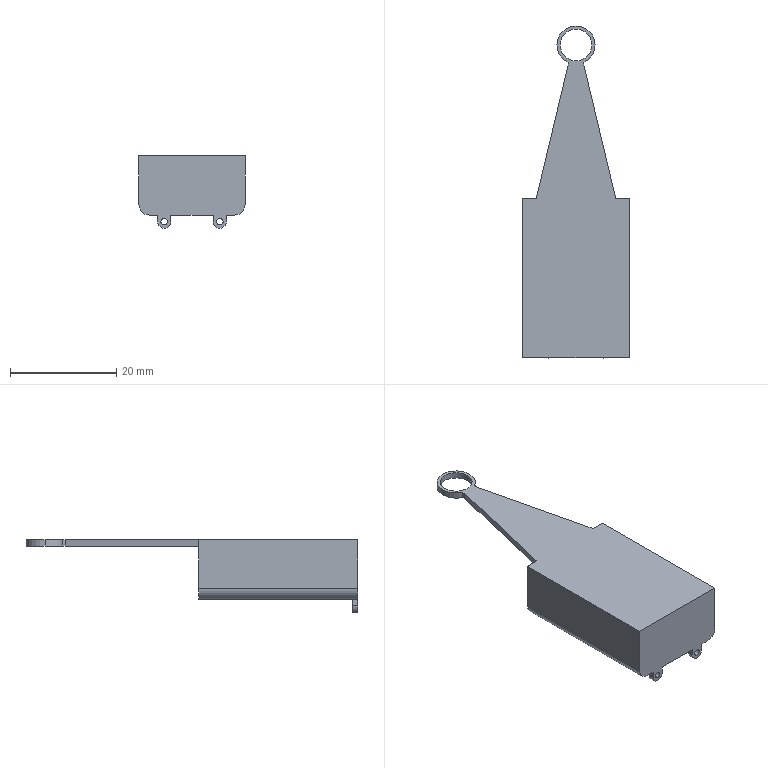Part | SolidWorks | features ICE 2, Extrusion 1, Fillet 1 | 1 solid | 32 faces | box 20 x 62.6 x 13.7 mm | volume 6966 mm3 | plane 17 | cylinder 15 | commonest cylinder face diameters 1.2 x4 2.5 x4 7.2 x3 4 x2 6 x2
STEP:
#1=CARTESIAN_POINT('',(5.25,1.,-6.25));
#2=VERTEX_POINT('',#1);
#3=CARTESIAN_POINT('',(5.25,1.,-7.45));
#4=VERTEX_POINT('',#3);
#5=CARTESIAN_POINT('',(5.25,1.,-6.85));
#6=DIRECTION('',(0.,-1.,0.));
#7=DIRECTION('',(0.,0.,1.));
#8=AXIS2_PLACEMENT_3D('',#5,#6,#7);
#9=CIRCLE('',#8,0.6);
#10=EDGE_CURVE('',#2,#4,#9,.T.);
#11=ORIENTED_EDGE('',*,*,#10,.F.);
#12=CARTESIAN_POINT('',(5.25,0.,-6.25));
#13=VERTEX_POINT('',#12);
#14=CARTESIAN_POINT('',(5.25,1.,-6.25));
#15=DIRECTION('',(0.,-1.,0.));
#16=VECTOR('',#15,1000.);
#17=LINE('',#14,#16);
#18=EDGE_CURVE('',#2,#13,#17,.T.);
#19=ORIENTED_EDGE('',*,*,#18,.T.);
#20=CARTESIAN_POINT('',(5.25,0.,-7.45));
#21=VERTEX_POINT('',#20);
#22=CARTESIAN_POINT('',(5.25,0.,-6.85));
#23=DIRECTION('',(0.,-1.,0.));
#24=DIRECTION('',(0.,0.,1.));
#25=AXIS2_PLACEMENT_3D('',#22,#23,#24);
#26=CIRCLE('',#25,0.6);
#27=EDGE_CURVE('',#13,#21,#26,.T.);
#28=ORIENTED_EDGE('',*,*,#27,.T.);
#29=CARTESIAN_POINT('',(5.25,1.,-7.45));
#30=DIRECTION('',(0.,-1.,0.));
#31=VECTOR('',#30,1000.);
#32=LINE('',#29,#31);
#33=EDGE_CURVE('',#4,#21,#32,.T.);
#34=ORIENTED_EDGE('',*,*,#33,.F.);
#35=EDGE_LOOP('',(#11,#19,#28,#34));
#36=FACE_OUTER_BOUND('',#35,.T.);
#37=CARTESIAN_POINT('',(5.25,1.,-6.85));
#38=DIRECTION('',(0.,-1.,0.));
#39=DIRECTION('',(0.,0.,-1.));
#40=AXIS2_PLACEMENT_3D('',#37,#38,#39);
#41=CYLINDRICAL_SURFACE('',#40,0.6);
#42=ADVANCED_FACE('',(#36),#41,.F.);
#43=CARTESIAN_POINT('',(4.,1.,-6.85));
#44=VERTEX_POINT('',#43);
#45=CARTESIAN_POINT('',(5.25,1.,-8.1));
#46=VERTEX_POINT('',#45);
#47=CARTESIAN_POINT('',(5.25,1.,-6.85));
#48=DIRECTION('',(0.,-1.,0.));
#49=DIRECTION('',(0.,0.,1.));
#50=AXIS2_PLACEMENT_3D('',#47,#48,#49);
#51=CIRCLE('',#50,1.25);
#52=EDGE_CURVE('',#44,#46,#51,.T.);
#53=ORIENTED_EDGE('',*,*,#52,.T.);
#54=CARTESIAN_POINT('',(5.25,0.,-8.1));
#55=VERTEX_POINT('',#54);
#56=CARTESIAN_POINT('',(5.25,1.,-8.1));
#57=DIRECTION('',(0.,-1.,0.));
#58=VECTOR('',#57,1000.);
#59=LINE('',#56,#58);
#60=EDGE_CURVE('',#46,#55,#59,.T.);
#61=ORIENTED_EDGE('',*,*,#60,.T.);
#62=CARTESIAN_POINT('',(4.,0.,-6.85));
#63=VERTEX_POINT('',#62);
#64=CARTESIAN_POINT('',(5.25,0.,-6.85));
#65=DIRECTION('',(0.,-1.,0.));
#66=DIRECTION('',(0.,0.,1.));
#67=AXIS2_PLACEMENT_3D('',#64,#65,#66);
#68=CIRCLE('',#67,1.25);
#69=EDGE_CURVE('',#63,#55,#68,.T.);
#70=ORIENTED_EDGE('',*,*,#69,.F.);
#71=CARTESIAN_POINT('',(4.,1.,-6.85));
#72=DIRECTION('',(0.,-1.,0.));
#73=VECTOR('',#72,1000.);
#74=LINE('',#71,#73);
#75=EDGE_CURVE('',#44,#63,#74,.T.);
#76=ORIENTED_EDGE('',*,*,#75,.F.);
#77=EDGE_LOOP('',(#53,#61,#70,#76));
#78=FACE_OUTER_BOUND('',#77,.T.);
#79=CARTESIAN_POINT('',(5.25,1.,-6.85));
#80=DIRECTION('',(0.,-1.,0.));
#81=DIRECTION('',(0.,0.,-1.));
#82=AXIS2_PLACEMENT_3D('',#79,#80,#81);
#83=CYLINDRICAL_SURFACE('',#82,1.25);
#84=ADVANCED_FACE('',(#78),#83,.T.);
#85=CARTESIAN_POINT('',(-5.25,1.,-6.25));
#86=VERTEX_POINT('',#85);
#87=CARTESIAN_POINT('',(-5.25,1.,-7.45));
#88=VERTEX_POINT('',#87);
#89=CARTESIAN_POINT('',(-5.25,1.,-6.85));
#90=DIRECTION('',(0.,-1.,0.));
#91=DIRECTION('',(0.,0.,-1.));
#92=AXIS2_PLACEMENT_3D('',#89,#90,#91);
#93=CIRCLE('',#92,0.6);
#94=EDGE_CURVE('',#86,#88,#93,.T.);
#95=ORIENTED_EDGE('',*,*,#94,.F.);
#96=CARTESIAN_POINT('',(-5.25,0.,-6.25));
#97=VERTEX_POINT('',#96);
#98=CARTESIAN_POINT('',(-5.25,1.,-6.25));
#99=DIRECTION('',(0.,-1.,0.));
#100=VECTOR('',#99,1000.);
#101=LINE('',#98,#100);
#102=EDGE_CURVE('',#86,#97,#101,.T.);
#103=ORIENTED_EDGE('',*,*,#102,.T.);
#104=CARTESIAN_POINT('',(-5.25,0.,-7.45));
#105=VERTEX_POINT('',#104);
#106=CARTESIAN_POINT('',(-5.25,0.,-6.85));
#107=DIRECTION('',(0.,-1.,0.));
#108=DIRECTION('',(0.,0.,-1.));
#109=AXIS2_PLACEMENT_3D('',#106,#107,#108);
#110=CIRCLE('',#109,0.6);
#111=EDGE_CURVE('',#97,#105,#110,.T.);
#112=ORIENTED_EDGE('',*,*,#111,.T.);
#113=CARTESIAN_POINT('',(-5.25,1.,-7.45));
#114=DIRECTION('',(0.,-1.,0.));
#115=VECTOR('',#114,1000.);
#116=LINE('',#113,#115);
#117=EDGE_CURVE('',#88,#105,#116,.T.);
#118=ORIENTED_EDGE('',*,*,#117,.F.);
#119=EDGE_LOOP('',(#95,#103,#112,#118));
#120=FACE_OUTER_BOUND('',#119,.T.);
#121=CARTESIAN_POINT('',(-5.25,1.,-6.85));
#122=DIRECTION('',(0.,-1.,0.));
#123=DIRECTION('',(0.,0.,-1.));
#124=AXIS2_PLACEMENT_3D('',#121,#122,#123);
#125=CYLINDRICAL_SURFACE('',#124,0.6);
#126=ADVANCED_FACE('',(#120),#125,.F.);
#127=CARTESIAN_POINT('',(-6.5,1.,-6.85));
#128=VERTEX_POINT('',#127);
#129=CARTESIAN_POINT('',(-5.25,1.,-8.1));
#130=VERTEX_POINT('',#129);
#131=CARTESIAN_POINT('',(-5.25,1.,-6.85));
#132=DIRECTION('',(0.,-1.,0.));
#133=DIRECTION('',(0.,0.,-1.));
#134=AXIS2_PLACEMENT_3D('',#131,#132,#133);
#135=CIRCLE('',#134,1.25);
#136=EDGE_CURVE('',#128,#130,#135,.T.);
#137=ORIENTED_EDGE('',*,*,#136,.T.);
#138=CARTESIAN_POINT('',(-5.25,0.,-8.1));
#139=VERTEX_POINT('',#138);
#140=CARTESIAN_POINT('',(-5.25,1.,-8.1));
#141=DIRECTION('',(0.,-1.,0.));
#142=VECTOR('',#141,1000.);
#143=LINE('',#140,#142);
#144=EDGE_CURVE('',#130,#139,#143,.T.);
#145=ORIENTED_EDGE('',*,*,#144,.T.);
#146=CARTESIAN_POINT('',(-6.5,0.,-6.85));
#147=VERTEX_POINT('',#146);
#148=CARTESIAN_POINT('',(-5.25,0.,-6.85));
#149=DIRECTION('',(0.,-1.,0.));
#150=DIRECTION('',(0.,0.,-1.));
#151=AXIS2_PLACEMENT_3D('',#148,#149,#150);
#152=CIRCLE('',#151,1.25);
#153=EDGE_CURVE('',#147,#139,#152,.T.);
#154=ORIENTED_EDGE('',*,*,#153,.F.);
#155=CARTESIAN_POINT('',(-6.5,1.,-6.85));
#156=DIRECTION('',(0.,-1.,0.));
#157=VECTOR('',#156,1000.);
#158=LINE('',#155,#157);
#159=EDGE_CURVE('',#128,#147,#158,.T.);
#160=ORIENTED_EDGE('',*,*,#159,.F.);
#161=EDGE_LOOP('',(#137,#145,#154,#160));
#162=FACE_OUTER_BOUND('',#161,.T.);
#163=CARTESIAN_POINT('',(-5.25,1.,-6.85));
#164=DIRECTION('',(0.,-1.,0.));
#165=DIRECTION('',(0.,0.,-1.));
#166=AXIS2_PLACEMENT_3D('',#163,#164,#165);
#167=CYLINDRICAL_SURFACE('',#166,1.25);
#168=ADVANCED_FACE('',(#162),#167,.T.);
#169=CARTESIAN_POINT('',(-3.,59.,4.4));
#170=VERTEX_POINT('',#169);
#171=CARTESIAN_POINT('',(3.,59.,4.4));
#172=VERTEX_POINT('',#171);
#173=CARTESIAN_POINT('',(0.,59.,4.4));
#174=DIRECTION('',(0.,0.,1.));
#175=DIRECTION('',(1.,0.,0.));
#176=AXIS2_PLACEMENT_3D('',#173,#174,#175);
#177=CIRCLE('',#176,3.);
#178=EDGE_CURVE('',#170,#172,#177,.T.);
#179=ORIENTED_EDGE('',*,*,#178,.F.);
#180=CARTESIAN_POINT('',(-3.,59.,5.6));
#181=VERTEX_POINT('',#180);
#182=CARTESIAN_POINT('',(-3.,59.,4.4));
#183=DIRECTION('',(0.,0.,1.));
#184=VECTOR('',#183,1000.);
#185=LINE('',#182,#184);
#186=EDGE_CURVE('',#170,#181,#185,.T.);
#187=ORIENTED_EDGE('',*,*,#186,.T.);
#188=CARTESIAN_POINT('',(3.,59.,5.6));
#189=VERTEX_POINT('',#188);
#190=CARTESIAN_POINT('',(0.,59.,5.6));
#191=DIRECTION('',(0.,0.,1.));
#192=DIRECTION('',(1.,0.,0.));
#193=AXIS2_PLACEMENT_3D('',#190,#191,#192);
#194=CIRCLE('',#193,3.);
#195=EDGE_CURVE('',#181,#189,#194,.T.);
#196=ORIENTED_EDGE('',*,*,#195,.T.);
#197=CARTESIAN_POINT('',(3.,59.,4.4));
#198=DIRECTION('',(0.,0.,1.));
#199=VECTOR('',#198,1000.);
#200=LINE('',#197,#199);
#201=EDGE_CURVE('',#172,#189,#200,.T.);
#202=ORIENTED_EDGE('',*,*,#201,.F.);
#203=EDGE_LOOP('',(#179,#187,#196,#202));
#204=FACE_OUTER_BOUND('',#203,.T.);
#205=CARTESIAN_POINT('',(0.,59.,4.4));
#206=DIRECTION('',(0.,0.,1.));
#207=DIRECTION('',(1.,0.,0.));
#208=AXIS2_PLACEMENT_3D('',#205,#206,#207);
#209=CYLINDRICAL_SURFACE('',#208,3.);
#210=ADVANCED_FACE('',(#204),#209,.F.);
#211=CARTESIAN_POINT('',(3.6,59.,4.4));
#212=VERTEX_POINT('',#211);
#213=CARTESIAN_POINT('',(-3.6,59.,4.4));
#214=VERTEX_POINT('',#213);
#215=CARTESIAN_POINT('',(0.,59.,4.4));
#216=DIRECTION('',(0.,0.,1.));
#217=DIRECTION('',(1.,0.,0.));
#218=AXIS2_PLACEMENT_3D('',#215,#216,#217);
#219=CIRCLE('',#218,3.6);
#220=EDGE_CURVE('',#212,#214,#219,.T.);
#221=ORIENTED_EDGE('',*,*,#220,.T.);
#222=CARTESIAN_POINT('',(-3.6,59.,5.6));
#223=VERTEX_POINT('',#222);
#224=CARTESIAN_POINT('',(-3.6,59.,4.4));
#225=DIRECTION('',(0.,0.,1.));
#226=VECTOR('',#225,1000.);
#227=LINE('',#224,#226);
#228=EDGE_CURVE('',#214,#223,#227,.T.);
#229=ORIENTED_EDGE('',*,*,#228,.T.);
#230=CARTESIAN_POINT('',(3.6,59.,5.6));
#231=VERTEX_POINT('',#230);
#232=CARTESIAN_POINT('',(0.,59.,5.6));
#233=DIRECTION('',(0.,0.,1.));
#234=DIRECTION('',(1.,0.,0.));
#235=AXIS2_PLACEMENT_3D('',#232,#233,#234);
#236=CIRCLE('',#235,3.6);
#237=EDGE_CURVE('',#231,#223,#236,.T.);
#238=ORIENTED_EDGE('',*,*,#237,.F.);
#239=CARTESIAN_POINT('',(3.6,59.,4.4));
#240=DIRECTION('',(0.,0.,1.));
#241=VECTOR('',#240,1000.);
#242=LINE('',#239,#241);
#243=EDGE_CURVE('',#212,#231,#242,.T.);
#244=ORIENTED_EDGE('',*,*,#243,.F.);
#245=EDGE_LOOP('',(#221,#229,#238,#244));
#246=FACE_OUTER_BOUND('',#245,.T.);
#247=CARTESIAN_POINT('',(0.,59.,4.4));
#248=DIRECTION('',(0.,0.,1.));
#249=DIRECTION('',(1.,0.,0.));
#250=AXIS2_PLACEMENT_3D('',#247,#248,#249);
#251=CYLINDRICAL_SURFACE('',#250,3.6);
#252=ADVANCED_FACE('',(#246),#251,.T.);
#253=CARTESIAN_POINT('',(1.5,55.727,4.4));
#254=VERTEX_POINT('',#253);
#255=CARTESIAN_POINT('',(0.,59.,4.4));
#256=DIRECTION('',(0.,0.,1.));
#257=DIRECTION('',(1.,0.,0.));
#258=AXIS2_PLACEMENT_3D('',#255,#256,#257);
#259=CIRCLE('',#258,3.6);
#260=EDGE_CURVE('',#254,#212,#259,.T.);
#261=ORIENTED_EDGE('',*,*,#260,.T.);
#262=ORIENTED_EDGE('',*,*,#243,.T.);
#263=CARTESIAN_POINT('',(1.5,55.727,5.6));
#264=VERTEX_POINT('',#263);
#265=CARTESIAN_POINT('',(0.,59.,5.6));
#266=DIRECTION('',(0.,0.,1.));
#267=DIRECTION('',(1.,0.,0.));
#268=AXIS2_PLACEMENT_3D('',#265,#266,#267);
#269=CIRCLE('',#268,3.6);
#270=EDGE_CURVE('',#264,#231,#269,.T.);
#271=ORIENTED_EDGE('',*,*,#270,.F.);
#272=CARTESIAN_POINT('',(1.5,55.727,4.4));
#273=DIRECTION('',(0.,0.,1.));
#274=VECTOR('',#273,1000.);
#275=LINE('',#272,#274);
#276=EDGE_CURVE('',#254,#264,#275,.T.);
#277=ORIENTED_EDGE('',*,*,#276,.F.);
#278=EDGE_LOOP('',(#261,#262,#271,#277));
#279=FACE_OUTER_BOUND('',#278,.T.);
#280=CARTESIAN_POINT('',(0.,59.,4.4));
#281=DIRECTION('',(0.,0.,1.));
#282=DIRECTION('',(1.,0.,0.));
#283=AXIS2_PLACEMENT_3D('',#280,#281,#282);
#284=CYLINDRICAL_SURFACE('',#283,3.6);
#285=ADVANCED_FACE('',(#279),#284,.T.);
#286=CARTESIAN_POINT('',(10.,0.,5.6));
#287=VERTEX_POINT('',#286);
#288=CARTESIAN_POINT('',(10.,0.,-3.6));
#289=VERTEX_POINT('',#288);
#290=CARTESIAN_POINT('',(10.,0.,-5.6));
#291=DIRECTION('',(0.,0.,-1.));
#292=VECTOR('',#291,1000.);
#293=LINE('',#290,#292);
#294=EDGE_CURVE('',#287,#289,#293,.T.);
#295=ORIENTED_EDGE('',*,*,#294,.T.);
#296=CARTESIAN_POINT('',(10.,30.,-3.6));
#297=VERTEX_POINT('',#296);
#298=CARTESIAN_POINT('',(10.,30.,-3.6));
#299=DIRECTION('',(0.,1.,0.));
#300=VECTOR('',#299,1000.);
#301=LINE('',#298,#300);
#302=EDGE_CURVE('',#289,#297,#301,.T.);
#303=ORIENTED_EDGE('',*,*,#302,.T.);
#304=CARTESIAN_POINT('',(10.,30.,5.6));
#305=VERTEX_POINT('',#304);
#306=CARTESIAN_POINT('',(10.,30.,-5.6));
#307=DIRECTION('',(0.,0.,-1.));
#308=VECTOR('',#307,1000.);
#309=LINE('',#306,#308);
#310=EDGE_CURVE('',#305,#297,#309,.T.);
#311=ORIENTED_EDGE('',*,*,#310,.F.);
#312=CARTESIAN_POINT('',(10.,30.,5.6));
#313=DIRECTION('',(0.,-1.,0.));
#314=VECTOR('',#313,1000.);
#315=LINE('',#312,#314);
#316=EDGE_CURVE('',#305,#287,#315,.T.);
#317=ORIENTED_EDGE('',*,*,#316,.T.);
#318=EDGE_LOOP('',(#295,#303,#311,#317));
#319=FACE_OUTER_BOUND('',#318,.T.);
#320=CARTESIAN_POINT('',(10.,30.,-5.6));
#321=DIRECTION('',(-1.,0.,0.));
#322=DIRECTION('',(0.,0.,1.));
#323=AXIS2_PLACEMENT_3D('',#320,#321,#322);
#324=PLANE('',#323);
#325=ADVANCED_FACE('',(#319),#324,.F.);
#326=CARTESIAN_POINT('',(8.,0.,-5.6));
#327=VERTEX_POINT('',#326);
#328=CARTESIAN_POINT('',(6.5,0.,-5.6));
#329=VERTEX_POINT('',#328);
#330=CARTESIAN_POINT('',(-10.,0.,-5.6));
#331=DIRECTION('',(-1.,0.,0.));
#332=VECTOR('',#331,1000.);
#333=LINE('',#330,#332);
#334=EDGE_CURVE('',#327,#329,#333,.T.);
#335=ORIENTED_EDGE('',*,*,#334,.T.);
#336=CARTESIAN_POINT('',(6.5,1.,-5.6));
#337=VERTEX_POINT('',#336);
#338=CARTESIAN_POINT('',(6.5,1.,-5.6));
#339=DIRECTION('',(0.,-1.,0.));
#340=VECTOR('',#339,1000.);
#341=LINE('',#338,#340);
#342=EDGE_CURVE('',#337,#329,#341,.T.);
#343=ORIENTED_EDGE('',*,*,#342,.F.);
#344=CARTESIAN_POINT('',(4.,1.,-5.6));
#345=VERTEX_POINT('',#344);
#346=CARTESIAN_POINT('',(6.5,1.,-5.6));
#347=DIRECTION('',(-1.,0.,0.));
#348=VECTOR('',#347,1000.);
#349=LINE('',#346,#348);
#350=EDGE_CURVE('',#337,#345,#349,.T.);
#351=ORIENTED_EDGE('',*,*,#350,.T.);
#352=CARTESIAN_POINT('',(4.,0.,-5.6));
#353=VERTEX_POINT('',#352);
#354=CARTESIAN_POINT('',(4.,1.,-5.6));
#355=DIRECTION('',(0.,-1.,0.));
#356=VECTOR('',#355,1000.);
#357=LINE('',#354,#356);
#358=EDGE_CURVE('',#345,#353,#357,.T.);
#359=ORIENTED_EDGE('',*,*,#358,.T.);
#360=CARTESIAN_POINT('',(-4.,0.,-5.6));
#361=VERTEX_POINT('',#360);
#362=CARTESIAN_POINT('',(-10.,0.,-5.6));
#363=DIRECTION('',(-1.,0.,0.));
#364=VECTOR('',#363,1000.);
#365=LINE('',#362,#364);
#366=EDGE_CURVE('',#353,#361,#365,.T.);
#367=ORIENTED_EDGE('',*,*,#366,.T.);
#368=CARTESIAN_POINT('',(-4.,1.,-5.6));
#369=VERTEX_POINT('',#368);
#370=CARTESIAN_POINT('',(-4.,1.,-5.6));
#371=DIRECTION('',(0.,-1.,0.));
#372=VECTOR('',#371,1000.);
#373=LINE('',#370,#372);
#374=EDGE_CURVE('',#369,#361,#373,.T.);
#375=ORIENTED_EDGE('',*,*,#374,.F.);
#376=CARTESIAN_POINT('',(-6.5,1.,-5.6));
#377=VERTEX_POINT('',#376);
#378=CARTESIAN_POINT('',(-6.5,1.,-5.6));
#379=DIRECTION('',(-1.,0.,0.));
#380=VECTOR('',#379,1000.);
#381=LINE('',#378,#380);
#382=EDGE_CURVE('',#369,#377,#381,.T.);
#383=ORIENTED_EDGE('',*,*,#382,.T.);
#384=CARTESIAN_POINT('',(-6.5,0.,-5.6));
#385=VERTEX_POINT('',#384);
#386=CARTESIAN_POINT('',(-6.5,1.,-5.6));
#387=DIRECTION('',(0.,-1.,0.));
#388=VECTOR('',#387,1000.);
#389=LINE('',#386,#388);
#390=EDGE_CURVE('',#377,#385,#389,.T.);
#391=ORIENTED_EDGE('',*,*,#390,.T.);
#392=CARTESIAN_POINT('',(-8.,0.,-5.6));
#393=VERTEX_POINT('',#392);
#394=CARTESIAN_POINT('',(-10.,0.,-5.6));
#395=DIRECTION('',(-1.,0.,0.));
#396=VECTOR('',#395,1000.);
#397=LINE('',#394,#396);
#398=EDGE_CURVE('',#385,#393,#397,.T.);
#399=ORIENTED_EDGE('',*,*,#398,.T.);
#400=CARTESIAN_POINT('',(-8.,30.,-5.6));
#401=VERTEX_POINT('',#400);
#402=CARTESIAN_POINT('',(-8.,30.,-5.6));
#403=DIRECTION('',(0.,1.,0.));
#404=VECTOR('',#403,1000.);
#405=LINE('',#402,#404);
#406=EDGE_CURVE('',#393,#401,#405,.T.);
#407=ORIENTED_EDGE('',*,*,#406,.T.);
#408=CARTESIAN_POINT('',(8.,30.,-5.6));
#409=VERTEX_POINT('',#408);
#410=CARTESIAN_POINT('',(-10.,30.,-5.6));
#411=DIRECTION('',(-1.,0.,0.));
#412=VECTOR('',#411,1000.);
#413=LINE('',#410,#412);
#414=EDGE_CURVE('',#409,#401,#413,.T.);
#415=ORIENTED_EDGE('',*,*,#414,.F.);
#416=CARTESIAN_POINT('',(8.,30.,-5.6));
#417=DIRECTION('',(0.,-1.,0.));
#418=VECTOR('',#417,1000.);
#419=LINE('',#416,#418);
#420=EDGE_CURVE('',#409,#327,#419,.T.);
#421=ORIENTED_EDGE('',*,*,#420,.T.);
#422=EDGE_LOOP('',(#335,#343,#351,#359,#367,#375,#383,#391,#399,#407,#415,#421));
#423=FACE_OUTER_BOUND('',#422,.T.);
#424=CARTESIAN_POINT('',(-10.,30.,-5.6));
#425=DIRECTION('',(0.,0.,1.));
#426=DIRECTION('',(1.,0.,0.));
#427=AXIS2_PLACEMENT_3D('',#424,#425,#426);
#428=PLANE('',#427);
#429=ADVANCED_FACE('',(#423),#428,.F.);
#430=CARTESIAN_POINT('',(-10.,30.,-3.6));
#431=VERTEX_POINT('',#430);
#432=CARTESIAN_POINT('',(-10.,30.,5.6));
#433=VERTEX_POINT('',#432);
#434=CARTESIAN_POINT('',(-10.,30.,-5.6));
#435=DIRECTION('',(0.,0.,1.));
#436=VECTOR('',#435,1000.);
#437=LINE('',#434,#436);
#438=EDGE_CURVE('',#431,#433,#437,.T.);
#439=ORIENTED_EDGE('',*,*,#438,.F.);
#440=CARTESIAN_POINT('',(-10.,0.,-3.6));
#441=VERTEX_POINT('',#440);
#442=CARTESIAN_POINT('',(-10.,30.,-3.6));
#443=DIRECTION('',(0.,-1.,0.));
#444=VECTOR('',#443,1000.);
#445=LINE('',#442,#444);
#446=EDGE_CURVE('',#431,#441,#445,.T.);
#447=ORIENTED_EDGE('',*,*,#446,.T.);
#448=CARTESIAN_POINT('',(-10.,0.,5.6));
#449=VERTEX_POINT('',#448);
#450=CARTESIAN_POINT('',(-10.,0.,-5.6));
#451=DIRECTION('',(0.,0.,1.));
#452=VECTOR('',#451,1000.);
#453=LINE('',#450,#452);
#454=EDGE_CURVE('',#441,#449,#453,.T.);
#455=ORIENTED_EDGE('',*,*,#454,.T.);
#456=CARTESIAN_POINT('',(-10.,30.,5.6));
#457=DIRECTION('',(0.,-1.,0.));
#458=VECTOR('',#457,1000.);
#459=LINE('',#456,#458);
#460=EDGE_CURVE('',#433,#449,#459,.T.);
#461=ORIENTED_EDGE('',*,*,#460,.F.);
#462=EDGE_LOOP('',(#439,#447,#455,#461));
#463=FACE_OUTER_BOUND('',#462,.T.);
#464=CARTESIAN_POINT('',(-10.,30.,-5.6));
#465=DIRECTION('',(1.,0.,0.));
#466=DIRECTION('',(0.,0.,-1.));
#467=AXIS2_PLACEMENT_3D('',#464,#465,#466);
#468=PLANE('',#467);
#469=ADVANCED_FACE('',(#463),#468,.F.);
#470=CARTESIAN_POINT('',(-10.,0.,5.6));
#471=DIRECTION('',(1.,0.,0.));
#472=VECTOR('',#471,1000.);
#473=LINE('',#470,#472);
#474=EDGE_CURVE('',#449,#287,#473,.T.);
#475=ORIENTED_EDGE('',*,*,#474,.T.);
#476=ORIENTED_EDGE('',*,*,#316,.F.);
#477=CARTESIAN_POINT('',(7.5,30.,5.6));
#478=VERTEX_POINT('',#477);
#479=CARTESIAN_POINT('',(-10.,30.,5.6));
#480=DIRECTION('',(1.,0.,0.));
#481=VECTOR('',#480,1000.);
#482=LINE('',#479,#481);
#483=EDGE_CURVE('',#478,#305,#482,.T.);
#484=ORIENTED_EDGE('',*,*,#483,.F.);
#485=CARTESIAN_POINT('',(1.5,55.197,5.6));
#486=VERTEX_POINT('',#485);
#487=CARTESIAN_POINT('',(1.5,55.197,5.6));
#488=DIRECTION('',(-0.2316,0.9728,0.));
#489=VECTOR('',#488,1000.);
#490=LINE('',#487,#489);
#491=EDGE_CURVE('',#478,#486,#490,.T.);
#492=ORIENTED_EDGE('',*,*,#491,.T.);
#493=CARTESIAN_POINT('',(1.5,55.727,5.6));
#494=DIRECTION('',(0.,1.,0.));
#495=VECTOR('',#494,1000.);
#496=LINE('',#493,#495);
#497=EDGE_CURVE('',#486,#264,#496,.T.);
#498=ORIENTED_EDGE('',*,*,#497,.T.);
#499=ORIENTED_EDGE('',*,*,#270,.T.);
#500=ORIENTED_EDGE('',*,*,#237,.T.);
#501=CARTESIAN_POINT('',(-1.5,55.727,5.6));
#502=VERTEX_POINT('',#501);
#503=CARTESIAN_POINT('',(0.,59.,5.6));
#504=DIRECTION('',(0.,0.,1.));
#505=DIRECTION('',(1.,0.,0.));
#506=AXIS2_PLACEMENT_3D('',#503,#504,#505);
#507=CIRCLE('',#506,3.6);
#508=EDGE_CURVE('',#223,#502,#507,.T.);
#509=ORIENTED_EDGE('',*,*,#508,.T.);
#510=CARTESIAN_POINT('',(-1.5,55.197,5.6));
#511=VERTEX_POINT('',#510);
#512=CARTESIAN_POINT('',(-1.5,55.727,5.6));
#513=DIRECTION('',(0.,-1.,0.));
#514=VECTOR('',#513,1000.);
#515=LINE('',#512,#514);
#516=EDGE_CURVE('',#502,#511,#515,.T.);
#517=ORIENTED_EDGE('',*,*,#516,.T.);
#518=CARTESIAN_POINT('',(-7.5,30.,5.6));
#519=VERTEX_POINT('',#518);
#520=CARTESIAN_POINT('',(-1.5,55.197,5.6));
#521=DIRECTION('',(-0.2316,-0.9728,0.));
#522=VECTOR('',#521,1000.);
#523=LINE('',#520,#522);
#524=EDGE_CURVE('',#511,#519,#523,.T.);
#525=ORIENTED_EDGE('',*,*,#524,.T.);
#526=CARTESIAN_POINT('',(-10.,30.,5.6));
#527=DIRECTION('',(1.,0.,0.));
#528=VECTOR('',#527,1000.);
#529=LINE('',#526,#528);
#530=EDGE_CURVE('',#433,#519,#529,.T.);
#531=ORIENTED_EDGE('',*,*,#530,.F.);
#532=ORIENTED_EDGE('',*,*,#460,.T.);
#533=EDGE_LOOP('',(#475,#476,#484,#492,#498,#499,#500,#509,#517,#525,#531,#532));
#534=FACE_OUTER_BOUND('',#533,.T.);
#535=CARTESIAN_POINT('',(0.,59.,5.6));
#536=DIRECTION('',(0.,0.,1.));
#537=DIRECTION('',(1.,0.,0.));
#538=AXIS2_PLACEMENT_3D('',#535,#536,#537);
#539=CIRCLE('',#538,3.);
#540=EDGE_CURVE('',#189,#181,#539,.T.);
#541=ORIENTED_EDGE('',*,*,#540,.F.);
#542=ORIENTED_EDGE('',*,*,#195,.F.);
#543=EDGE_LOOP('',(#541,#542));
#544=FACE_BOUND('',#543,.T.);
#545=CARTESIAN_POINT('',(-10.,30.,5.6));
#546=DIRECTION('',(0.,0.,-1.));
#547=DIRECTION('',(-1.,0.,0.));
#548=AXIS2_PLACEMENT_3D('',#545,#546,#547);
#549=PLANE('',#548);
#550=ADVANCED_FACE('',(#534,#544),#549,.F.);
#551=ORIENTED_EDGE('',*,*,#414,.T.);
#552=CARTESIAN_POINT('',(-8.,30.,-3.6));
#553=DIRECTION('',(0.,1.,0.));
#554=DIRECTION('',(0.,0.,1.));
#555=AXIS2_PLACEMENT_3D('',#552,#553,#554);
#556=CIRCLE('',#555,2.);
#557=EDGE_CURVE('',#401,#431,#556,.T.);
#558=ORIENTED_EDGE('',*,*,#557,.T.);
#559=ORIENTED_EDGE('',*,*,#438,.T.);
#560=ORIENTED_EDGE('',*,*,#530,.T.);
#561=CARTESIAN_POINT('',(-7.5,30.,4.4));
#562=VERTEX_POINT('',#561);
#563=CARTESIAN_POINT('',(-7.5,30.,4.4));
#564=DIRECTION('',(0.,0.,1.));
#565=VECTOR('',#564,1000.);
#566=LINE('',#563,#565);
#567=EDGE_CURVE('',#562,#519,#566,.T.);
#568=ORIENTED_EDGE('',*,*,#567,.F.);
#569=CARTESIAN_POINT('',(7.5,30.,4.4));
#570=VERTEX_POINT('',#569);
#571=CARTESIAN_POINT('',(7.5,30.,4.4));
#572=DIRECTION('',(1.,0.,0.));
#573=VECTOR('',#572,1000.);
#574=LINE('',#571,#573);
#575=EDGE_CURVE('',#562,#570,#574,.T.);
#576=ORIENTED_EDGE('',*,*,#575,.T.);
#577=CARTESIAN_POINT('',(7.5,30.,4.4));
#578=DIRECTION('',(0.,0.,1.));
#579=VECTOR('',#578,1000.);
#580=LINE('',#577,#579);
#581=EDGE_CURVE('',#570,#478,#580,.T.);
#582=ORIENTED_EDGE('',*,*,#581,.T.);
#583=ORIENTED_EDGE('',*,*,#483,.T.);
#584=ORIENTED_EDGE('',*,*,#310,.T.);
#585=CARTESIAN_POINT('',(8.,30.,-3.6));
#586=DIRECTION('',(0.,1.,0.));
#587=DIRECTION('',(0.,0.,1.));
#588=AXIS2_PLACEMENT_3D('',#585,#586,#587);
#589=CIRCLE('',#588,2.);
#590=EDGE_CURVE('',#297,#409,#589,.T.);
#591=ORIENTED_EDGE('',*,*,#590,.T.);
#592=EDGE_LOOP('',(#551,#558,#559,#560,#568,#576,#582,#583,#584,#591));
#593=FACE_OUTER_BOUND('',#592,.T.);
#594=CARTESIAN_POINT('',(0.,30.,0.));
#595=DIRECTION('',(0.,1.,0.));
#596=DIRECTION('',(0.,0.,1.));
#597=AXIS2_PLACEMENT_3D('',#594,#595,#596);
#598=PLANE('',#597);
#599=ADVANCED_FACE('',(#593),#598,.T.);
#600=ORIENTED_EDGE('',*,*,#454,.F.);
#601=CARTESIAN_POINT('',(-8.,0.,-3.6));
#602=DIRECTION('',(0.,-1.,0.));
#603=DIRECTION('',(0.,0.,1.));
#604=AXIS2_PLACEMENT_3D('',#601,#602,#603);
#605=CIRCLE('',#604,2.);
#606=EDGE_CURVE('',#441,#393,#605,.T.);
#607=ORIENTED_EDGE('',*,*,#606,.T.);
#608=ORIENTED_EDGE('',*,*,#398,.F.);
#609=CARTESIAN_POINT('',(-6.5,0.,-5.6));
#610=DIRECTION('',(0.,0.,-1.));
#611=VECTOR('',#610,1000.);
#612=LINE('',#609,#611);
#613=EDGE_CURVE('',#385,#147,#612,.T.);
#614=ORIENTED_EDGE('',*,*,#613,.T.);
#615=ORIENTED_EDGE('',*,*,#153,.T.);
#616=CARTESIAN_POINT('',(-4.,0.,-6.85));
#617=VERTEX_POINT('',#616);
#618=CARTESIAN_POINT('',(-5.25,0.,-6.85));
#619=DIRECTION('',(0.,-1.,0.));
#620=DIRECTION('',(0.,0.,-1.));
#621=AXIS2_PLACEMENT_3D('',#618,#619,#620);
#622=CIRCLE('',#621,1.25);
#623=EDGE_CURVE('',#139,#617,#622,.T.);
#624=ORIENTED_EDGE('',*,*,#623,.T.);
#625=CARTESIAN_POINT('',(-4.,0.,-5.6));
#626=DIRECTION('',(0.,0.,1.));
#627=VECTOR('',#626,1000.);
#628=LINE('',#625,#627);
#629=EDGE_CURVE('',#617,#361,#628,.T.);
#630=ORIENTED_EDGE('',*,*,#629,.T.);
#631=ORIENTED_EDGE('',*,*,#366,.F.);
#632=CARTESIAN_POINT('',(4.,0.,-5.6));
#633=DIRECTION('',(0.,0.,-1.));
#634=VECTOR('',#633,1000.);
#635=LINE('',#632,#634);
#636=EDGE_CURVE('',#353,#63,#635,.T.);
#637=ORIENTED_EDGE('',*,*,#636,.T.);
#638=ORIENTED_EDGE('',*,*,#69,.T.);
#639=CARTESIAN_POINT('',(6.5,0.,-6.85));
#640=VERTEX_POINT('',#639);
#641=CARTESIAN_POINT('',(5.25,0.,-6.85));
#642=DIRECTION('',(0.,-1.,0.));
#643=DIRECTION('',(0.,0.,1.));
#644=AXIS2_PLACEMENT_3D('',#641,#642,#643);
#645=CIRCLE('',#644,1.25);
#646=EDGE_CURVE('',#55,#640,#645,.T.);
#647=ORIENTED_EDGE('',*,*,#646,.T.);
#648=CARTESIAN_POINT('',(6.5,0.,-5.6));
#649=DIRECTION('',(0.,0.,1.));
#650=VECTOR('',#649,1000.);
#651=LINE('',#648,#650);
#652=EDGE_CURVE('',#640,#329,#651,.T.);
#653=ORIENTED_EDGE('',*,*,#652,.T.);
#654=ORIENTED_EDGE('',*,*,#334,.F.);
#655=CARTESIAN_POINT('',(8.,0.,-3.6));
#656=DIRECTION('',(0.,-1.,0.));
#657=DIRECTION('',(0.,0.,1.));
#658=AXIS2_PLACEMENT_3D('',#655,#656,#657);
#659=CIRCLE('',#658,2.);
#660=EDGE_CURVE('',#327,#289,#659,.T.);
#661=ORIENTED_EDGE('',*,*,#660,.T.);
#662=ORIENTED_EDGE('',*,*,#294,.F.);
#663=ORIENTED_EDGE('',*,*,#474,.F.);
#664=EDGE_LOOP('',(#600,#607,#608,#614,#615,#624,#630,#631,#637,#638,#647,#653,#654,#661,#662,#663));
#665=FACE_OUTER_BOUND('',#664,.T.);
#666=CARTESIAN_POINT('',(-5.25,0.,-6.85));
#667=DIRECTION('',(0.,-1.,0.));
#668=DIRECTION('',(0.,0.,-1.));
#669=AXIS2_PLACEMENT_3D('',#666,#667,#668);
#670=CIRCLE('',#669,0.6);
#671=EDGE_CURVE('',#105,#97,#670,.T.);
#672=ORIENTED_EDGE('',*,*,#671,.F.);
#673=ORIENTED_EDGE('',*,*,#111,.F.);
#674=EDGE_LOOP('',(#672,#673));
#675=FACE_BOUND('',#674,.T.);
#676=CARTESIAN_POINT('',(5.25,0.,-6.85));
#677=DIRECTION('',(0.,-1.,0.));
#678=DIRECTION('',(0.,0.,1.));
#679=AXIS2_PLACEMENT_3D('',#676,#677,#678);
#680=CIRCLE('',#679,0.6);
#681=EDGE_CURVE('',#21,#13,#680,.T.);
#682=ORIENTED_EDGE('',*,*,#681,.F.);
#683=ORIENTED_EDGE('',*,*,#27,.F.);
#684=EDGE_LOOP('',(#682,#683));
#685=FACE_BOUND('',#684,.T.);
#686=CARTESIAN_POINT('',(0.,0.,0.));
#687=DIRECTION('',(0.,1.,0.));
#688=DIRECTION('',(0.,0.,1.));
#689=AXIS2_PLACEMENT_3D('',#686,#687,#688);
#690=PLANE('',#689);
#691=ADVANCED_FACE('',(#665,#675,#685),#690,.F.);
#692=ORIENTED_EDGE('',*,*,#516,.F.);
#693=CARTESIAN_POINT('',(-1.5,55.727,4.4));
#694=VERTEX_POINT('',#693);
#695=CARTESIAN_POINT('',(-1.5,55.727,4.4));
#696=DIRECTION('',(0.,0.,1.));
#697=VECTOR('',#696,1000.);
#698=LINE('',#695,#697);
#699=EDGE_CURVE('',#694,#502,#698,.T.);
#700=ORIENTED_EDGE('',*,*,#699,.F.);
#701=CARTESIAN_POINT('',(-1.5,55.197,4.4));
#702=VERTEX_POINT('',#701);
#703=CARTESIAN_POINT('',(-1.5,55.727,4.4));
#704=DIRECTION('',(0.,-1.,0.));
#705=VECTOR('',#704,1000.);
#706=LINE('',#703,#705);
#707=EDGE_CURVE('',#694,#702,#706,.T.);
#708=ORIENTED_EDGE('',*,*,#707,.T.);
#709=CARTESIAN_POINT('',(-1.5,55.197,4.4));
#710=DIRECTION('',(0.,0.,1.));
#711=VECTOR('',#710,1000.);
#712=LINE('',#709,#711);
#713=EDGE_CURVE('',#702,#511,#712,.T.);
#714=ORIENTED_EDGE('',*,*,#713,.T.);
#715=EDGE_LOOP('',(#692,#700,#708,#714));
#716=FACE_OUTER_BOUND('',#715,.T.);
#717=CARTESIAN_POINT('',(-1.5,55.727,4.4));
#718=DIRECTION('',(-1.,0.,0.));
#719=DIRECTION('',(0.,0.,1.));
#720=AXIS2_PLACEMENT_3D('',#717,#718,#719);
#721=PLANE('',#720);
#722=ADVANCED_FACE('',(#716),#721,.T.);
#723=ORIENTED_EDGE('',*,*,#228,.F.);
#724=CARTESIAN_POINT('',(0.,59.,4.4));
#725=DIRECTION('',(0.,0.,1.));
#726=DIRECTION('',(1.,0.,0.));
#727=AXIS2_PLACEMENT_3D('',#724,#725,#726);
#728=CIRCLE('',#727,3.6);
#729=EDGE_CURVE('',#214,#694,#728,.T.);
#730=ORIENTED_EDGE('',*,*,#729,.T.);
#731=ORIENTED_EDGE('',*,*,#699,.T.);
#732=ORIENTED_EDGE('',*,*,#508,.F.);
#733=EDGE_LOOP('',(#723,#730,#731,#732));
#734=FACE_OUTER_BOUND('',#733,.T.);
#735=CARTESIAN_POINT('',(0.,59.,4.4));
#736=DIRECTION('',(0.,0.,1.));
#737=DIRECTION('',(1.,0.,0.));
#738=AXIS2_PLACEMENT_3D('',#735,#736,#737);
#739=CYLINDRICAL_SURFACE('',#738,3.6);
#740=ADVANCED_FACE('',(#734),#739,.T.);
#741=ORIENTED_EDGE('',*,*,#497,.F.);
#742=CARTESIAN_POINT('',(1.5,55.197,4.4));
#743=VERTEX_POINT('',#742);
#744=CARTESIAN_POINT('',(1.5,55.197,4.4));
#745=DIRECTION('',(0.,0.,1.));
#746=VECTOR('',#745,1000.);
#747=LINE('',#744,#746);
#748=EDGE_CURVE('',#743,#486,#747,.T.);
#749=ORIENTED_EDGE('',*,*,#748,.F.);
#750=CARTESIAN_POINT('',(1.5,55.727,4.4));
#751=DIRECTION('',(0.,1.,0.));
#752=VECTOR('',#751,1000.);
#753=LINE('',#750,#752);
#754=EDGE_CURVE('',#743,#254,#753,.T.);
#755=ORIENTED_EDGE('',*,*,#754,.T.);
#756=ORIENTED_EDGE('',*,*,#276,.T.);
#757=EDGE_LOOP('',(#741,#749,#755,#756));
#758=FACE_OUTER_BOUND('',#757,.T.);
#759=CARTESIAN_POINT('',(1.5,55.727,4.4));
#760=DIRECTION('',(1.,0.,0.));
#761=DIRECTION('',(0.,0.,-1.));
#762=AXIS2_PLACEMENT_3D('',#759,#760,#761);
#763=PLANE('',#762);
#764=ADVANCED_FACE('',(#758),#763,.T.);
#765=ORIENTED_EDGE('',*,*,#491,.F.);
#766=ORIENTED_EDGE('',*,*,#581,.F.);
#767=CARTESIAN_POINT('',(1.5,55.197,4.4));
#768=DIRECTION('',(-0.2316,0.9728,0.));
#769=VECTOR('',#768,1000.);
#770=LINE('',#767,#769);
#771=EDGE_CURVE('',#570,#743,#770,.T.);
#772=ORIENTED_EDGE('',*,*,#771,.T.);
#773=ORIENTED_EDGE('',*,*,#748,.T.);
#774=EDGE_LOOP('',(#765,#766,#772,#773));
#775=FACE_OUTER_BOUND('',#774,.T.);
#776=CARTESIAN_POINT('',(1.5,55.197,4.4));
#777=DIRECTION('',(0.9728,0.2316,0.));
#778=DIRECTION('',(-0.2316,0.9728,0.));
#779=AXIS2_PLACEMENT_3D('',#776,#777,#778);
#780=PLANE('',#779);
#781=ADVANCED_FACE('',(#775),#780,.T.);
#782=ORIENTED_EDGE('',*,*,#524,.F.);
#783=ORIENTED_EDGE('',*,*,#713,.F.);
#784=CARTESIAN_POINT('',(-1.5,55.197,4.4));
#785=DIRECTION('',(-0.2316,-0.9728,0.));
#786=VECTOR('',#785,1000.);
#787=LINE('',#784,#786);
#788=EDGE_CURVE('',#702,#562,#787,.T.);
#789=ORIENTED_EDGE('',*,*,#788,.T.);
#790=ORIENTED_EDGE('',*,*,#567,.T.);
#791=EDGE_LOOP('',(#782,#783,#789,#790));
#792=FACE_OUTER_BOUND('',#791,.T.);
#793=CARTESIAN_POINT('',(-1.5,55.197,4.4));
#794=DIRECTION('',(-0.9728,0.2316,0.));
#795=DIRECTION('',(-0.2316,-0.9728,0.));
#796=AXIS2_PLACEMENT_3D('',#793,#794,#795);
#797=PLANE('',#796);
#798=ADVANCED_FACE('',(#792),#797,.T.);
#799=CARTESIAN_POINT('',(0.,59.,4.4));
#800=DIRECTION('',(0.,0.,1.));
#801=DIRECTION('',(1.,0.,0.));
#802=AXIS2_PLACEMENT_3D('',#799,#800,#801);
#803=CIRCLE('',#802,3.);
#804=EDGE_CURVE('',#172,#170,#803,.T.);
#805=ORIENTED_EDGE('',*,*,#804,.T.);
#806=ORIENTED_EDGE('',*,*,#178,.T.);
#807=EDGE_LOOP('',(#805,#806));
#808=FACE_BOUND('',#807,.T.);
#809=ORIENTED_EDGE('',*,*,#707,.F.);
#810=ORIENTED_EDGE('',*,*,#729,.F.);
#811=ORIENTED_EDGE('',*,*,#220,.F.);
#812=ORIENTED_EDGE('',*,*,#260,.F.);
#813=ORIENTED_EDGE('',*,*,#754,.F.);
#814=ORIENTED_EDGE('',*,*,#771,.F.);
#815=ORIENTED_EDGE('',*,*,#575,.F.);
#816=ORIENTED_EDGE('',*,*,#788,.F.);
#817=EDGE_LOOP('',(#809,#810,#811,#812,#813,#814,#815,#816));
#818=FACE_OUTER_BOUND('',#817,.T.);
#819=CARTESIAN_POINT('',(0.,59.,4.4));
#820=DIRECTION('',(0.,0.,1.));
#821=DIRECTION('',(1.,0.,0.));
#822=AXIS2_PLACEMENT_3D('',#819,#820,#821);
#823=PLANE('',#822);
#824=ADVANCED_FACE('',(#808,#818),#823,.F.);
#825=ORIENTED_EDGE('',*,*,#186,.F.);
#826=ORIENTED_EDGE('',*,*,#804,.F.);
#827=ORIENTED_EDGE('',*,*,#201,.T.);
#828=ORIENTED_EDGE('',*,*,#540,.T.);
#829=EDGE_LOOP('',(#825,#826,#827,#828));
#830=FACE_OUTER_BOUND('',#829,.T.);
#831=CARTESIAN_POINT('',(0.,59.,4.4));
#832=DIRECTION('',(0.,0.,1.));
#833=DIRECTION('',(1.,0.,0.));
#834=AXIS2_PLACEMENT_3D('',#831,#832,#833);
#835=CYLINDRICAL_SURFACE('',#834,3.);
#836=ADVANCED_FACE('',(#830),#835,.F.);
#837=ORIENTED_EDGE('',*,*,#557,.F.);
#838=ORIENTED_EDGE('',*,*,#406,.F.);
#839=ORIENTED_EDGE('',*,*,#606,.F.);
#840=ORIENTED_EDGE('',*,*,#446,.F.);
#841=EDGE_LOOP('',(#837,#838,#839,#840));
#842=FACE_OUTER_BOUND('',#841,.T.);
#843=CARTESIAN_POINT('',(-8.,30.,-3.6));
#844=DIRECTION('',(0.,-1.,0.));
#845=DIRECTION('',(0.,0.,-1.));
#846=AXIS2_PLACEMENT_3D('',#843,#844,#845);
#847=CYLINDRICAL_SURFACE('',#846,2.);
#848=ADVANCED_FACE('',(#842),#847,.T.);
#849=ORIENTED_EDGE('',*,*,#590,.F.);
#850=ORIENTED_EDGE('',*,*,#302,.F.);
#851=ORIENTED_EDGE('',*,*,#660,.F.);
#852=ORIENTED_EDGE('',*,*,#420,.F.);
#853=EDGE_LOOP('',(#849,#850,#851,#852));
#854=FACE_OUTER_BOUND('',#853,.T.);
#855=CARTESIAN_POINT('',(8.,30.,-3.6));
#856=DIRECTION('',(0.,-1.,0.));
#857=DIRECTION('',(0.,0.,-1.));
#858=AXIS2_PLACEMENT_3D('',#855,#856,#857);
#859=CYLINDRICAL_SURFACE('',#858,2.);
#860=ADVANCED_FACE('',(#854),#859,.T.);
#861=ORIENTED_EDGE('',*,*,#613,.F.);
#862=ORIENTED_EDGE('',*,*,#390,.F.);
#863=CARTESIAN_POINT('',(-6.5,1.,-5.6));
#864=DIRECTION('',(0.,0.,-1.));
#865=VECTOR('',#864,1000.);
#866=LINE('',#863,#865);
#867=EDGE_CURVE('',#377,#128,#866,.T.);
#868=ORIENTED_EDGE('',*,*,#867,.T.);
#869=ORIENTED_EDGE('',*,*,#159,.T.);
#870=EDGE_LOOP('',(#861,#862,#868,#869));
#871=FACE_OUTER_BOUND('',#870,.T.);
#872=CARTESIAN_POINT('',(-6.5,1.,-5.6));
#873=DIRECTION('',(-1.,0.,0.));
#874=DIRECTION('',(0.,0.,1.));
#875=AXIS2_PLACEMENT_3D('',#872,#873,#874);
#876=PLANE('',#875);
#877=ADVANCED_FACE('',(#871),#876,.T.);
#878=ORIENTED_EDGE('',*,*,#629,.F.);
#879=CARTESIAN_POINT('',(-4.,1.,-6.85));
#880=VERTEX_POINT('',#879);
#881=CARTESIAN_POINT('',(-4.,1.,-6.85));
#882=DIRECTION('',(0.,-1.,0.));
#883=VECTOR('',#882,1000.);
#884=LINE('',#881,#883);
#885=EDGE_CURVE('',#880,#617,#884,.T.);
#886=ORIENTED_EDGE('',*,*,#885,.F.);
#887=CARTESIAN_POINT('',(-4.,1.,-5.6));
#888=DIRECTION('',(0.,0.,1.));
#889=VECTOR('',#888,1000.);
#890=LINE('',#887,#889);
#891=EDGE_CURVE('',#880,#369,#890,.T.);
#892=ORIENTED_EDGE('',*,*,#891,.T.);
#893=ORIENTED_EDGE('',*,*,#374,.T.);
#894=EDGE_LOOP('',(#878,#886,#892,#893));
#895=FACE_OUTER_BOUND('',#894,.T.);
#896=CARTESIAN_POINT('',(-4.,1.,-5.6));
#897=DIRECTION('',(1.,0.,0.));
#898=DIRECTION('',(0.,0.,-1.));
#899=AXIS2_PLACEMENT_3D('',#896,#897,#898);
#900=PLANE('',#899);
#901=ADVANCED_FACE('',(#895),#900,.T.);
#902=ORIENTED_EDGE('',*,*,#144,.F.);
#903=CARTESIAN_POINT('',(-5.25,1.,-6.85));
#904=DIRECTION('',(0.,-1.,0.));
#905=DIRECTION('',(0.,0.,-1.));
#906=AXIS2_PLACEMENT_3D('',#903,#904,#905);
#907=CIRCLE('',#906,1.25);
#908=EDGE_CURVE('',#130,#880,#907,.T.);
#909=ORIENTED_EDGE('',*,*,#908,.T.);
#910=ORIENTED_EDGE('',*,*,#885,.T.);
#911=ORIENTED_EDGE('',*,*,#623,.F.);
#912=EDGE_LOOP('',(#902,#909,#910,#911));
#913=FACE_OUTER_BOUND('',#912,.T.);
#914=CARTESIAN_POINT('',(-5.25,1.,-6.85));
#915=DIRECTION('',(0.,-1.,0.));
#916=DIRECTION('',(0.,0.,-1.));
#917=AXIS2_PLACEMENT_3D('',#914,#915,#916);
#918=CYLINDRICAL_SURFACE('',#917,1.25);
#919=ADVANCED_FACE('',(#913),#918,.T.);
#920=CARTESIAN_POINT('',(-5.25,1.,-6.85));
#921=DIRECTION('',(0.,-1.,0.));
#922=DIRECTION('',(0.,0.,-1.));
#923=AXIS2_PLACEMENT_3D('',#920,#921,#922);
#924=CIRCLE('',#923,0.6);
#925=EDGE_CURVE('',#88,#86,#924,.T.);
#926=ORIENTED_EDGE('',*,*,#925,.T.);
#927=ORIENTED_EDGE('',*,*,#94,.T.);
#928=EDGE_LOOP('',(#926,#927));
#929=FACE_BOUND('',#928,.T.);
#930=ORIENTED_EDGE('',*,*,#867,.F.);
#931=ORIENTED_EDGE('',*,*,#382,.F.);
#932=ORIENTED_EDGE('',*,*,#891,.F.);
#933=ORIENTED_EDGE('',*,*,#908,.F.);
#934=ORIENTED_EDGE('',*,*,#136,.F.);
#935=EDGE_LOOP('',(#930,#931,#932,#933,#934));
#936=FACE_OUTER_BOUND('',#935,.T.);
#937=CARTESIAN_POINT('',(-5.25,1.,-6.85));
#938=DIRECTION('',(0.,-1.,0.));
#939=DIRECTION('',(0.,0.,-1.));
#940=AXIS2_PLACEMENT_3D('',#937,#938,#939);
#941=PLANE('',#940);
#942=ADVANCED_FACE('',(#929,#936),#941,.F.);
#943=ORIENTED_EDGE('',*,*,#102,.F.);
#944=ORIENTED_EDGE('',*,*,#925,.F.);
#945=ORIENTED_EDGE('',*,*,#117,.T.);
#946=ORIENTED_EDGE('',*,*,#671,.T.);
#947=EDGE_LOOP('',(#943,#944,#945,#946));
#948=FACE_OUTER_BOUND('',#947,.T.);
#949=CARTESIAN_POINT('',(-5.25,1.,-6.85));
#950=DIRECTION('',(0.,-1.,0.));
#951=DIRECTION('',(0.,0.,-1.));
#952=AXIS2_PLACEMENT_3D('',#949,#950,#951);
#953=CYLINDRICAL_SURFACE('',#952,0.6);
#954=ADVANCED_FACE('',(#948),#953,.F.);
#955=ORIENTED_EDGE('',*,*,#652,.F.);
#956=CARTESIAN_POINT('',(6.5,1.,-6.85));
#957=VERTEX_POINT('',#956);
#958=CARTESIAN_POINT('',(6.5,1.,-6.85));
#959=DIRECTION('',(0.,-1.,0.));
#960=VECTOR('',#959,1000.);
#961=LINE('',#958,#960);
#962=EDGE_CURVE('',#957,#640,#961,.T.);
#963=ORIENTED_EDGE('',*,*,#962,.F.);
#964=CARTESIAN_POINT('',(6.5,1.,-5.6));
#965=DIRECTION('',(0.,0.,1.));
#966=VECTOR('',#965,1000.);
#967=LINE('',#964,#966);
#968=EDGE_CURVE('',#957,#337,#967,.T.);
#969=ORIENTED_EDGE('',*,*,#968,.T.);
#970=ORIENTED_EDGE('',*,*,#342,.T.);
#971=EDGE_LOOP('',(#955,#963,#969,#970));
#972=FACE_OUTER_BOUND('',#971,.T.);
#973=CARTESIAN_POINT('',(6.5,1.,-5.6));
#974=DIRECTION('',(1.,0.,0.));
#975=DIRECTION('',(0.,0.,-1.));
#976=AXIS2_PLACEMENT_3D('',#973,#974,#975);
#977=PLANE('',#976);
#978=ADVANCED_FACE('',(#972),#977,.T.);
#979=ORIENTED_EDGE('',*,*,#60,.F.);
#980=CARTESIAN_POINT('',(5.25,1.,-6.85));
#981=DIRECTION('',(0.,-1.,0.));
#982=DIRECTION('',(0.,0.,1.));
#983=AXIS2_PLACEMENT_3D('',#980,#981,#982);
#984=CIRCLE('',#983,1.25);
#985=EDGE_CURVE('',#46,#957,#984,.T.);
#986=ORIENTED_EDGE('',*,*,#985,.T.);
#987=ORIENTED_EDGE('',*,*,#962,.T.);
#988=ORIENTED_EDGE('',*,*,#646,.F.);
#989=EDGE_LOOP('',(#979,#986,#987,#988));
#990=FACE_OUTER_BOUND('',#989,.T.);
#991=CARTESIAN_POINT('',(5.25,1.,-6.85));
#992=DIRECTION('',(0.,-1.,0.));
#993=DIRECTION('',(0.,0.,-1.));
#994=AXIS2_PLACEMENT_3D('',#991,#992,#993);
#995=CYLINDRICAL_SURFACE('',#994,1.25);
#996=ADVANCED_FACE('',(#990),#995,.T.);
#997=ORIENTED_EDGE('',*,*,#636,.F.);
#998=ORIENTED_EDGE('',*,*,#358,.F.);
#999=CARTESIAN_POINT('',(4.,1.,-5.6));
#1000=DIRECTION('',(0.,0.,-1.));
#1001=VECTOR('',#1000,1000.);
#1002=LINE('',#999,#1001);
#1003=EDGE_CURVE('',#345,#44,#1002,.T.);
#1004=ORIENTED_EDGE('',*,*,#1003,.T.);
#1005=ORIENTED_EDGE('',*,*,#75,.T.);
#1006=EDGE_LOOP('',(#997,#998,#1004,#1005));
#1007=FACE_OUTER_BOUND('',#1006,.T.);
#1008=CARTESIAN_POINT('',(4.,1.,-5.6));
#1009=DIRECTION('',(-1.,0.,0.));
#1010=DIRECTION('',(0.,0.,1.));
#1011=AXIS2_PLACEMENT_3D('',#1008,#1009,#1010);
#1012=PLANE('',#1011);
#1013=ADVANCED_FACE('',(#1007),#1012,.T.);
#1014=CARTESIAN_POINT('',(5.25,1.,-6.85));
#1015=DIRECTION('',(0.,-1.,0.));
#1016=DIRECTION('',(0.,0.,1.));
#1017=AXIS2_PLACEMENT_3D('',#1014,#1015,#1016);
#1018=CIRCLE('',#1017,0.6);
#1019=EDGE_CURVE('',#4,#2,#1018,.T.);
#1020=ORIENTED_EDGE('',*,*,#1019,.T.);
#1021=ORIENTED_EDGE('',*,*,#10,.T.);
#1022=EDGE_LOOP('',(#1020,#1021));
#1023=FACE_BOUND('',#1022,.T.);
#1024=ORIENTED_EDGE('',*,*,#968,.F.);
#1025=ORIENTED_EDGE('',*,*,#985,.F.);
#1026=ORIENTED_EDGE('',*,*,#52,.F.);
#1027=ORIENTED_EDGE('',*,*,#1003,.F.);
#1028=ORIENTED_EDGE('',*,*,#350,.F.);
#1029=EDGE_LOOP('',(#1024,#1025,#1026,#1027,#1028));
#1030=FACE_OUTER_BOUND('',#1029,.T.);
#1031=CARTESIAN_POINT('',(5.25,1.,-6.85));
#1032=DIRECTION('',(0.,1.,0.));
#1033=DIRECTION('',(0.,0.,1.));
#1034=AXIS2_PLACEMENT_3D('',#1031,#1032,#1033);
#1035=PLANE('',#1034);
#1036=ADVANCED_FACE('',(#1023,#1030),#1035,.T.);
#1037=ORIENTED_EDGE('',*,*,#18,.F.);
#1038=ORIENTED_EDGE('',*,*,#1019,.F.);
#1039=ORIENTED_EDGE('',*,*,#33,.T.);
#1040=ORIENTED_EDGE('',*,*,#681,.T.);
#1041=EDGE_LOOP('',(#1037,#1038,#1039,#1040));
#1042=FACE_OUTER_BOUND('',#1041,.T.);
#1043=CARTESIAN_POINT('',(5.25,1.,-6.85));
#1044=DIRECTION('',(0.,-1.,0.));
#1045=DIRECTION('',(0.,0.,-1.));
#1046=AXIS2_PLACEMENT_3D('',#1043,#1044,#1045);
#1047=CYLINDRICAL_SURFACE('',#1046,0.6);
#1048=ADVANCED_FACE('',(#1042),#1047,.F.);
#1049=CLOSED_SHELL('',(#42,#84,#126,#168,#210,#252,#285,#325,#429,#469,#550,#599,#691,#722,#740,#764,#781,#798,#824,#836,#848,#860,#877,#901,#919,#942,#954,#978,#996,#1013,#1036,#1048));
#1050=MANIFOLD_SOLID_BREP('',#1049);
#1051=CARTESIAN_POINT('',(0.,0.,0.));
#1052=DIRECTION('',(0.,0.,1.));
#1053=DIRECTION('',(1.,0.,0.));
#1054=AXIS2_PLACEMENT_3D('',#1051,#1052,#1053);
#1055=(LENGTH_UNIT()NAMED_UNIT(*)SI_UNIT(.MILLI.,.METRE.));
#1056=UNCERTAINTY_MEASURE_WITH_UNIT(LENGTH_MEASURE(0.00001),#1055,'','');
#1057=(NAMED_UNIT(*)PLANE_ANGLE_UNIT()SI_UNIT($,.RADIAN.));
#1058=(NAMED_UNIT(*)SI_UNIT($,.STERADIAN.)SOLID_ANGLE_UNIT());
#1059=(GEOMETRIC_REPRESENTATION_CONTEXT(3)GLOBAL_UNCERTAINTY_ASSIGNED_CONTEXT((#1056))GLOBAL_UNIT_ASSIGNED_CONTEXT((#1055,#1057,#1058))REPRESENTATION_CONTEXT('',''));
#1060=ADVANCED_BREP_SHAPE_REPRESENTATION('',(#1050,#1054),#1059);